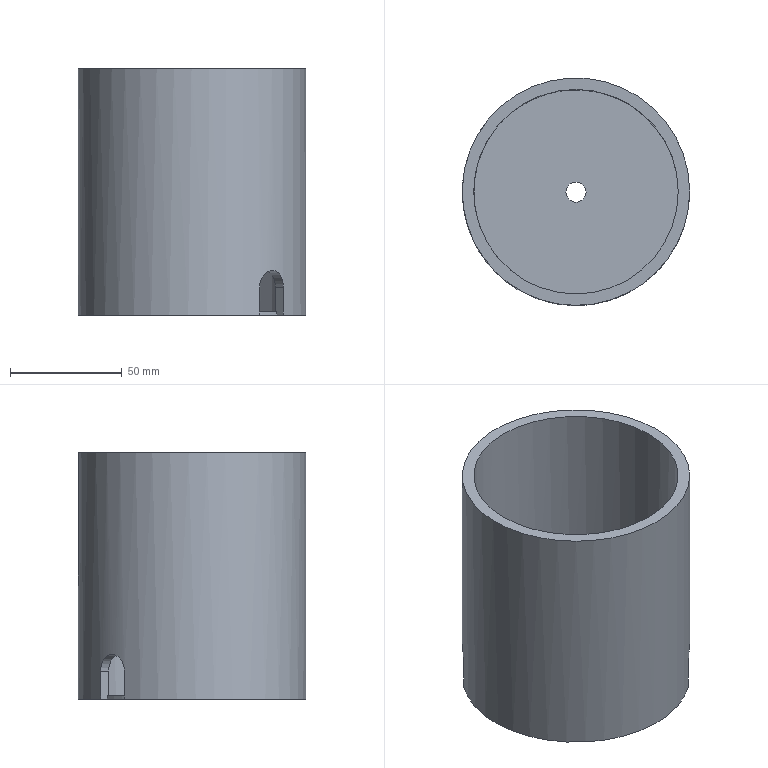Part | NX | features solid 2 | 1 solid | 14 faces | box 101.6 x 101.6 x 110 mm | volume 177690 mm3 | plane 7 | cylinder 7 | commonest cylinder face diameters 15 x2 93.2 x2 9 x1 91.4 x1 101.6 x1
STEP:
#1=CARTESIAN_POINT('',(-1547.218,877.825,-80.));
#2=VERTEX_POINT('',#1);
#3=CARTESIAN_POINT('',(-1550.224,880.831,-80.));
#4=VERTEX_POINT('',#3);
#5=CARTESIAN_POINT('',(-1458.128,788.735,-80.));
#6=DIRECTION('',(-0.7071,0.7071,0.));
#7=VECTOR('',#6,1000.);
#8=LINE('',#5,#7);
#9=EDGE_CURVE('',#2,#4,#8,.T.);
#10=ORIENTED_EDGE('',*,*,#9,.F.);
#11=CARTESIAN_POINT('',(-1547.218,877.825,-78.4));
#12=VERTEX_POINT('',#11);
#13=CARTESIAN_POINT('',(-1547.218,877.825,-78.4));
#14=DIRECTION('',(0.,0.,-1.));
#15=VECTOR('',#14,1000.);
#16=LINE('',#13,#15);
#17=EDGE_CURVE('',#2,#12,#16,.F.);
#18=ORIENTED_EDGE('',*,*,#17,.T.);
#19=CARTESIAN_POINT('',(-1546.573,877.18,-78.4));
#20=VERTEX_POINT('',#19);
#21=CARTESIAN_POINT('',(-1458.128,788.735,-78.4));
#22=DIRECTION('',(-0.7071,0.7071,0.));
#23=VECTOR('',#22,1000.);
#24=LINE('',#21,#23);
#25=EDGE_CURVE('',#20,#12,#24,.T.);
#26=ORIENTED_EDGE('',*,*,#25,.F.);
#27=CARTESIAN_POINT('',(-1546.573,877.18,-67.5));
#28=VERTEX_POINT('',#27);
#29=CARTESIAN_POINT('',(-1546.573,877.18,-80.));
#30=DIRECTION('',(0.,0.,1.));
#31=VECTOR('',#30,1000.);
#32=LINE('',#29,#31);
#33=EDGE_CURVE('',#28,#20,#32,.F.);
#34=ORIENTED_EDGE('',*,*,#33,.F.);
#35=CARTESIAN_POINT('',(-1550.224,880.831,-67.5));
#36=VERTEX_POINT('',#35);
#37=CARTESIAN_POINT('',(-1458.128,788.735,-67.5));
#38=DIRECTION('',(-0.7071,0.7071,0.));
#39=VECTOR('',#38,1000.);
#40=LINE('',#37,#39);
#41=EDGE_CURVE('',#28,#36,#40,.T.);
#42=ORIENTED_EDGE('',*,*,#41,.T.);
#43=CARTESIAN_POINT('',(-1550.224,880.831,-80.));
#44=DIRECTION('',(0.,0.,1.));
#45=VECTOR('',#44,1000.);
#46=LINE('',#43,#45);
#47=EDGE_CURVE('',#36,#4,#46,.F.);
#48=ORIENTED_EDGE('',*,*,#47,.T.);
#49=EDGE_LOOP('',(#10,#18,#26,#34,#42,#48));
#50=FACE_BOUND('',#49,.T.);
#51=CARTESIAN_POINT('',(-1458.128,788.735,-67.5));
#52=DIRECTION('',(-0.7071,-0.7071,0.));
#53=DIRECTION('',(0.,0.,1.));
#54=AXIS2_PLACEMENT_3D('',#51,#52,#53);
#55=PLANE('',#54);
#56=ADVANCED_FACE('',(#50),#55,.T.);
#57=CARTESIAN_POINT('',(-1557.825,867.218,-78.4));
#58=VERTEX_POINT('',#57);
#59=CARTESIAN_POINT('',(-1557.18,866.573,-78.4));
#60=VERTEX_POINT('',#59);
#61=CARTESIAN_POINT('',(-1468.735,778.128,-78.4));
#62=DIRECTION('',(0.7071,-0.7071,0.));
#63=VECTOR('',#62,1000.);
#64=LINE('',#61,#63);
#65=EDGE_CURVE('',#58,#60,#64,.T.);
#66=ORIENTED_EDGE('',*,*,#65,.F.);
#67=CARTESIAN_POINT('',(-1557.825,867.218,-80.));
#68=VERTEX_POINT('',#67);
#69=CARTESIAN_POINT('',(-1557.825,867.218,-78.4));
#70=DIRECTION('',(0.,0.,-1.));
#71=VECTOR('',#70,1000.);
#72=LINE('',#69,#71);
#73=EDGE_CURVE('',#58,#68,#72,.T.);
#74=ORIENTED_EDGE('',*,*,#73,.T.);
#75=CARTESIAN_POINT('',(-1560.831,870.224,-80.));
#76=VERTEX_POINT('',#75);
#77=CARTESIAN_POINT('',(-1468.735,778.128,-80.));
#78=DIRECTION('',(-0.7071,0.7071,0.));
#79=VECTOR('',#78,1000.);
#80=LINE('',#77,#79);
#81=EDGE_CURVE('',#68,#76,#80,.T.);
#82=ORIENTED_EDGE('',*,*,#81,.T.);
#83=CARTESIAN_POINT('',(-1560.831,870.224,-67.5));
#84=VERTEX_POINT('',#83);
#85=CARTESIAN_POINT('',(-1560.831,870.224,-80.));
#86=DIRECTION('',(0.,0.,1.));
#87=VECTOR('',#86,1000.);
#88=LINE('',#85,#87);
#89=EDGE_CURVE('',#76,#84,#88,.T.);
#90=ORIENTED_EDGE('',*,*,#89,.T.);
#91=CARTESIAN_POINT('',(-1557.18,866.573,-67.5));
#92=VERTEX_POINT('',#91);
#93=CARTESIAN_POINT('',(-1468.735,778.128,-67.5));
#94=DIRECTION('',(-0.7071,0.7071,0.));
#95=VECTOR('',#94,1000.);
#96=LINE('',#93,#95);
#97=EDGE_CURVE('',#92,#84,#96,.T.);
#98=ORIENTED_EDGE('',*,*,#97,.F.);
#99=CARTESIAN_POINT('',(-1557.18,866.573,-80.));
#100=DIRECTION('',(0.,0.,1.));
#101=VECTOR('',#100,1000.);
#102=LINE('',#99,#101);
#103=EDGE_CURVE('',#60,#92,#102,.T.);
#104=ORIENTED_EDGE('',*,*,#103,.F.);
#105=EDGE_LOOP('',(#66,#74,#82,#90,#98,#104));
#106=FACE_BOUND('',#105,.T.);
#107=CARTESIAN_POINT('',(-1468.735,778.128,-80.));
#108=DIRECTION('',(0.7071,0.7071,0.));
#109=DIRECTION('',(0.,0.,-1.));
#110=AXIS2_PLACEMENT_3D('',#107,#108,#109);
#111=PLANE('',#110);
#112=ADVANCED_FACE('',(#106),#111,.T.);
#113=CARTESIAN_POINT('',(-1489.776,799.169,-80.));
#114=VERTEX_POINT('',#113);
#115=CARTESIAN_POINT('',(-1492.782,802.175,-80.));
#116=VERTEX_POINT('',#115);
#117=CARTESIAN_POINT('',(-1468.735,778.128,-80.));
#118=DIRECTION('',(-0.7071,0.7071,0.));
#119=VECTOR('',#118,1000.);
#120=LINE('',#117,#119);
#121=EDGE_CURVE('',#114,#116,#120,.T.);
#122=ORIENTED_EDGE('',*,*,#121,.T.);
#123=CARTESIAN_POINT('',(-1492.782,802.175,-78.4));
#124=VERTEX_POINT('',#123);
#125=CARTESIAN_POINT('',(-1492.782,802.175,-78.4));
#126=DIRECTION('',(0.,0.,-1.));
#127=VECTOR('',#126,1000.);
#128=LINE('',#125,#127);
#129=EDGE_CURVE('',#116,#124,#128,.F.);
#130=ORIENTED_EDGE('',*,*,#129,.T.);
#131=CARTESIAN_POINT('',(-1493.427,802.82,-78.4));
#132=VERTEX_POINT('',#131);
#133=CARTESIAN_POINT('',(-1468.735,778.128,-78.4));
#134=DIRECTION('',(0.7071,-0.7071,0.));
#135=VECTOR('',#134,1000.);
#136=LINE('',#133,#135);
#137=EDGE_CURVE('',#132,#124,#136,.T.);
#138=ORIENTED_EDGE('',*,*,#137,.F.);
#139=CARTESIAN_POINT('',(-1493.427,802.82,-67.5));
#140=VERTEX_POINT('',#139);
#141=CARTESIAN_POINT('',(-1493.427,802.82,-80.));
#142=DIRECTION('',(0.,0.,1.));
#143=VECTOR('',#142,1000.);
#144=LINE('',#141,#143);
#145=EDGE_CURVE('',#140,#132,#144,.F.);
#146=ORIENTED_EDGE('',*,*,#145,.F.);
#147=CARTESIAN_POINT('',(-1489.776,799.169,-67.5));
#148=VERTEX_POINT('',#147);
#149=CARTESIAN_POINT('',(-1468.735,778.128,-67.5));
#150=DIRECTION('',(-0.7071,0.7071,0.));
#151=VECTOR('',#150,1000.);
#152=LINE('',#149,#151);
#153=EDGE_CURVE('',#148,#140,#152,.T.);
#154=ORIENTED_EDGE('',*,*,#153,.F.);
#155=CARTESIAN_POINT('',(-1489.776,799.169,-80.));
#156=DIRECTION('',(0.,0.,1.));
#157=VECTOR('',#156,1000.);
#158=LINE('',#155,#157);
#159=EDGE_CURVE('',#148,#114,#158,.F.);
#160=ORIENTED_EDGE('',*,*,#159,.T.);
#161=EDGE_LOOP('',(#122,#130,#138,#146,#154,#160));
#162=FACE_BOUND('',#161,.T.);
#163=CARTESIAN_POINT('',(-1468.735,778.128,-80.));
#164=DIRECTION('',(0.7071,0.7071,0.));
#165=DIRECTION('',(0.,0.,-1.));
#166=AXIS2_PLACEMENT_3D('',#163,#164,#165);
#167=PLANE('',#166);
#168=ADVANCED_FACE('',(#162),#167,.T.);
#169=CARTESIAN_POINT('',(-1482.175,812.782,-78.4));
#170=VERTEX_POINT('',#169);
#171=CARTESIAN_POINT('',(-1482.82,813.427,-78.4));
#172=VERTEX_POINT('',#171);
#173=CARTESIAN_POINT('',(-1458.128,788.735,-78.4));
#174=DIRECTION('',(-0.7071,0.7071,0.));
#175=VECTOR('',#174,1000.);
#176=LINE('',#173,#175);
#177=EDGE_CURVE('',#170,#172,#176,.T.);
#178=ORIENTED_EDGE('',*,*,#177,.F.);
#179=CARTESIAN_POINT('',(-1482.175,812.782,-80.));
#180=VERTEX_POINT('',#179);
#181=CARTESIAN_POINT('',(-1482.175,812.782,-78.4));
#182=DIRECTION('',(0.,0.,-1.));
#183=VECTOR('',#182,1000.);
#184=LINE('',#181,#183);
#185=EDGE_CURVE('',#170,#180,#184,.T.);
#186=ORIENTED_EDGE('',*,*,#185,.T.);
#187=CARTESIAN_POINT('',(-1479.169,809.776,-80.));
#188=VERTEX_POINT('',#187);
#189=CARTESIAN_POINT('',(-1458.128,788.735,-80.));
#190=DIRECTION('',(-0.7071,0.7071,0.));
#191=VECTOR('',#190,1000.);
#192=LINE('',#189,#191);
#193=EDGE_CURVE('',#188,#180,#192,.T.);
#194=ORIENTED_EDGE('',*,*,#193,.F.);
#195=CARTESIAN_POINT('',(-1479.169,809.776,-67.5));
#196=VERTEX_POINT('',#195);
#197=CARTESIAN_POINT('',(-1479.169,809.776,-80.));
#198=DIRECTION('',(0.,0.,1.));
#199=VECTOR('',#198,1000.);
#200=LINE('',#197,#199);
#201=EDGE_CURVE('',#188,#196,#200,.T.);
#202=ORIENTED_EDGE('',*,*,#201,.T.);
#203=CARTESIAN_POINT('',(-1482.82,813.427,-67.5));
#204=VERTEX_POINT('',#203);
#205=CARTESIAN_POINT('',(-1458.128,788.735,-67.5));
#206=DIRECTION('',(-0.7071,0.7071,0.));
#207=VECTOR('',#206,1000.);
#208=LINE('',#205,#207);
#209=EDGE_CURVE('',#196,#204,#208,.T.);
#210=ORIENTED_EDGE('',*,*,#209,.T.);
#211=CARTESIAN_POINT('',(-1482.82,813.427,-80.));
#212=DIRECTION('',(0.,0.,1.));
#213=VECTOR('',#212,1000.);
#214=LINE('',#211,#213);
#215=EDGE_CURVE('',#172,#204,#214,.T.);
#216=ORIENTED_EDGE('',*,*,#215,.F.);
#217=EDGE_LOOP('',(#178,#186,#194,#202,#210,#216));
#218=FACE_BOUND('',#217,.T.);
#219=CARTESIAN_POINT('',(-1458.128,788.735,-67.5));
#220=DIRECTION('',(-0.7071,-0.7071,0.));
#221=DIRECTION('',(0.,0.,1.));
#222=AXIS2_PLACEMENT_3D('',#219,#220,#221);
#223=PLANE('',#222);
#224=ADVANCED_FACE('',(#218),#223,.T.);
#225=CARTESIAN_POINT('',(-1515.5,840.,-80.));
#226=VERTEX_POINT('',#225);
#227=CARTESIAN_POINT('',(-1520.,840.,-80.));
#228=DIRECTION('',(0.,0.,-1.));
#229=DIRECTION('',(1.,0.,0.));
#230=AXIS2_PLACEMENT_3D('',#227,#228,#229);
#231=CIRCLE('',#230,4.5);
#232=EDGE_CURVE('',#226,#226,#231,.F.);
#233=ORIENTED_EDGE('',*,*,#232,.T.);
#234=EDGE_LOOP('',(#233));
#235=FACE_BOUND('',#234,.T.);
#236=CARTESIAN_POINT('',(-1520.,840.,-80.));
#237=DIRECTION('',(0.,0.,1.));
#238=DIRECTION('',(-1.,0.,0.));
#239=AXIS2_PLACEMENT_3D('',#236,#237,#238);
#240=CIRCLE('',#239,46.6);
#241=EDGE_CURVE('',#2,#68,#240,.T.);
#242=ORIENTED_EDGE('',*,*,#241,.F.);
#243=ORIENTED_EDGE('',*,*,#9,.T.);
#244=CARTESIAN_POINT('',(-1520.,840.,-80.));
#245=DIRECTION('',(0.,0.,-1.));
#246=DIRECTION('',(0.7071,0.7071,0.));
#247=AXIS2_PLACEMENT_3D('',#244,#245,#246);
#248=CIRCLE('',#247,50.8);
#249=EDGE_CURVE('',#4,#188,#248,.T.);
#250=ORIENTED_EDGE('',*,*,#249,.T.);
#251=ORIENTED_EDGE('',*,*,#193,.T.);
#252=CARTESIAN_POINT('',(-1520.,840.,-80.));
#253=DIRECTION('',(0.,0.,1.));
#254=DIRECTION('',(-1.,0.,0.));
#255=AXIS2_PLACEMENT_3D('',#252,#253,#254);
#256=CIRCLE('',#255,46.6);
#257=EDGE_CURVE('',#116,#180,#256,.T.);
#258=ORIENTED_EDGE('',*,*,#257,.F.);
#259=ORIENTED_EDGE('',*,*,#121,.F.);
#260=CARTESIAN_POINT('',(-1520.,840.,-80.));
#261=DIRECTION('',(0.,0.,-1.));
#262=DIRECTION('',(0.7071,0.7071,0.));
#263=AXIS2_PLACEMENT_3D('',#260,#261,#262);
#264=CIRCLE('',#263,50.8);
#265=EDGE_CURVE('',#114,#76,#264,.T.);
#266=ORIENTED_EDGE('',*,*,#265,.T.);
#267=ORIENTED_EDGE('',*,*,#81,.F.);
#268=EDGE_LOOP('',(#242,#243,#250,#251,#258,#259,#266,#267));
#269=FACE_BOUND('',#268,.T.);
#270=CARTESIAN_POINT('',(-1520.,840.,-80.));
#271=DIRECTION('',(0.,0.,-1.));
#272=DIRECTION('',(-0.7071,-0.7071,0.));
#273=AXIS2_PLACEMENT_3D('',#270,#271,#272);
#274=PLANE('',#273);
#275=ADVANCED_FACE('',(#235,#269),#274,.T.);
#276=CARTESIAN_POINT('',(-1474.3,840.,30.));
#277=VERTEX_POINT('',#276);
#278=CARTESIAN_POINT('',(-1520.,840.,30.));
#279=DIRECTION('',(0.,0.,-1.));
#280=DIRECTION('',(1.,0.,0.));
#281=AXIS2_PLACEMENT_3D('',#278,#279,#280);
#282=CIRCLE('',#281,45.7);
#283=EDGE_CURVE('',#277,#277,#282,.T.);
#284=ORIENTED_EDGE('',*,*,#283,.F.);
#285=EDGE_LOOP('',(#284));
#286=FACE_BOUND('',#285,.T.);
#287=ORIENTED_EDGE('',*,*,#33,.T.);
#288=CARTESIAN_POINT('',(-1520.,840.,-78.4));
#289=DIRECTION('',(0.,0.,1.));
#290=DIRECTION('',(-1.,0.,0.));
#291=AXIS2_PLACEMENT_3D('',#288,#289,#290);
#292=CIRCLE('',#291,45.7);
#293=EDGE_CURVE('',#20,#172,#292,.F.);
#294=ORIENTED_EDGE('',*,*,#293,.T.);
#295=ORIENTED_EDGE('',*,*,#215,.T.);
#296=CARTESIAN_POINT('',(-1493.427,802.82,-67.5));
#297=CARTESIAN_POINT('',(-1493.427,802.82,-65.54));
#298=CARTESIAN_POINT('',(-1492.058,803.748,-61.623));
#299=CARTESIAN_POINT('',(-1487.576,807.576,-59.188));
#300=CARTESIAN_POINT('',(-1483.745,812.061,-61.626));
#301=CARTESIAN_POINT('',(-1482.82,813.427,-65.541));
#302=CARTESIAN_POINT('',(-1482.82,813.427,-67.5));
#303=B_SPLINE_CURVE_WITH_KNOTS('',3,(#296,#297,#298,#299,#300,#301,#302),.UNSPECIFIED.,.F.,.F.,(4,1,1,1,4),(0.0344,0.04027,0.04614,0.05201,0.05788),.UNSPECIFIED.);
#304=EDGE_CURVE('',#140,#204,#303,.T.);
#305=ORIENTED_EDGE('',*,*,#304,.F.);
#306=ORIENTED_EDGE('',*,*,#145,.T.);
#307=CARTESIAN_POINT('',(-1520.,840.,-78.4));
#308=DIRECTION('',(0.,0.,1.));
#309=DIRECTION('',(-1.,0.,0.));
#310=AXIS2_PLACEMENT_3D('',#307,#308,#309);
#311=CIRCLE('',#310,45.7);
#312=EDGE_CURVE('',#132,#60,#311,.F.);
#313=ORIENTED_EDGE('',*,*,#312,.T.);
#314=ORIENTED_EDGE('',*,*,#103,.T.);
#315=CARTESIAN_POINT('',(-1546.573,877.18,-67.5));
#316=CARTESIAN_POINT('',(-1546.573,877.18,-65.54));
#317=CARTESIAN_POINT('',(-1547.942,876.252,-61.623));
#318=CARTESIAN_POINT('',(-1552.424,872.424,-59.188));
#319=CARTESIAN_POINT('',(-1556.255,867.939,-61.626));
#320=CARTESIAN_POINT('',(-1557.18,866.573,-65.541));
#321=CARTESIAN_POINT('',(-1557.18,866.573,-67.5));
#322=B_SPLINE_CURVE_WITH_KNOTS('',3,(#315,#316,#317,#318,#319,#320,#321),.UNSPECIFIED.,.F.,.F.,(4,1,1,1,4),(0.0344,0.04027,0.04614,0.05201,0.05788),.UNSPECIFIED.);
#323=EDGE_CURVE('',#28,#92,#322,.T.);
#324=ORIENTED_EDGE('',*,*,#323,.F.);
#325=EDGE_LOOP('',(#287,#294,#295,#305,#306,#313,#314,#324));
#326=FACE_BOUND('',#325,.T.);
#327=CARTESIAN_POINT('',(-1520.,840.,-80.));
#328=DIRECTION('',(0.,0.,1.));
#329=DIRECTION('',(0.7071,0.7071,0.));
#330=AXIS2_PLACEMENT_3D('',#327,#328,#329);
#331=CYLINDRICAL_SURFACE('',#330,45.7);
#332=ADVANCED_FACE('',(#286,#326),#331,.F.);
#333=ORIENTED_EDGE('',*,*,#201,.F.);
#334=ORIENTED_EDGE('',*,*,#249,.F.);
#335=ORIENTED_EDGE('',*,*,#47,.F.);
#336=CARTESIAN_POINT('',(-1550.224,880.831,-67.5));
#337=CARTESIAN_POINT('',(-1550.224,880.831,-65.515));
#338=CARTESIAN_POINT('',(-1551.571,879.879,-61.635));
#339=CARTESIAN_POINT('',(-1556.013,876.025,-59.184));
#340=CARTESIAN_POINT('',(-1559.879,871.572,-61.63));
#341=CARTESIAN_POINT('',(-1560.831,870.224,-65.515));
#342=CARTESIAN_POINT('',(-1560.831,870.224,-67.5));
#343=B_SPLINE_CURVE_WITH_KNOTS('',3,(#336,#337,#338,#339,#340,#341,#342),.UNSPECIFIED.,.F.,.F.,(4,1,1,1,4),(0.,0.005869,0.01174,0.01761,0.02347),.UNSPECIFIED.);
#344=EDGE_CURVE('',#36,#84,#343,.T.);
#345=ORIENTED_EDGE('',*,*,#344,.T.);
#346=ORIENTED_EDGE('',*,*,#89,.F.);
#347=ORIENTED_EDGE('',*,*,#265,.F.);
#348=ORIENTED_EDGE('',*,*,#159,.F.);
#349=CARTESIAN_POINT('',(-1489.776,799.169,-67.5));
#350=CARTESIAN_POINT('',(-1489.776,799.169,-65.515));
#351=CARTESIAN_POINT('',(-1488.429,800.121,-61.635));
#352=CARTESIAN_POINT('',(-1483.987,803.975,-59.184));
#353=CARTESIAN_POINT('',(-1480.121,808.428,-61.63));
#354=CARTESIAN_POINT('',(-1479.169,809.776,-65.515));
#355=CARTESIAN_POINT('',(-1479.169,809.776,-67.5));
#356=B_SPLINE_CURVE_WITH_KNOTS('',3,(#349,#350,#351,#352,#353,#354,#355),.UNSPECIFIED.,.F.,.F.,(4,1,1,1,4),(0.,0.005869,0.01174,0.01761,0.02347),.UNSPECIFIED.);
#357=EDGE_CURVE('',#148,#196,#356,.T.);
#358=ORIENTED_EDGE('',*,*,#357,.T.);
#359=EDGE_LOOP('',(#333,#334,#335,#345,#346,#347,#348,#358));
#360=FACE_BOUND('',#359,.T.);
#361=CARTESIAN_POINT('',(-1555.921,804.079,30.));
#362=VERTEX_POINT('',#361);
#363=CARTESIAN_POINT('',(-1520.,840.,30.));
#364=DIRECTION('',(0.,0.,1.));
#365=DIRECTION('',(-0.7071,-0.7071,0.));
#366=AXIS2_PLACEMENT_3D('',#363,#364,#365);
#367=CIRCLE('',#366,50.8);
#368=EDGE_CURVE('',#362,#362,#367,.F.);
#369=ORIENTED_EDGE('',*,*,#368,.T.);
#370=EDGE_LOOP('',(#369));
#371=FACE_BOUND('',#370,.T.);
#372=CARTESIAN_POINT('',(-1520.,840.,-80.));
#373=DIRECTION('',(0.,0.,1.));
#374=DIRECTION('',(0.7071,0.7071,0.));
#375=AXIS2_PLACEMENT_3D('',#372,#373,#374);
#376=CYLINDRICAL_SURFACE('',#375,50.8);
#377=ADVANCED_FACE('',(#360,#371),#376,.T.);
#378=ORIENTED_EDGE('',*,*,#283,.T.);
#379=EDGE_LOOP('',(#378));
#380=FACE_BOUND('',#379,.T.);
#381=ORIENTED_EDGE('',*,*,#368,.F.);
#382=EDGE_LOOP('',(#381));
#383=FACE_BOUND('',#382,.T.);
#384=CARTESIAN_POINT('',(-1520.,840.,30.));
#385=DIRECTION('',(0.,0.,-1.));
#386=DIRECTION('',(-0.7071,-0.7071,0.));
#387=AXIS2_PLACEMENT_3D('',#384,#385,#386);
#388=PLANE('',#387);
#389=ADVANCED_FACE('',(#380,#383),#388,.F.);
#390=ORIENTED_EDGE('',*,*,#41,.F.);
#391=ORIENTED_EDGE('',*,*,#323,.T.);
#392=ORIENTED_EDGE('',*,*,#97,.T.);
#393=ORIENTED_EDGE('',*,*,#344,.F.);
#394=EDGE_LOOP('',(#390,#391,#392,#393));
#395=FACE_BOUND('',#394,.T.);
#396=CARTESIAN_POINT('',(-1463.431,783.431,-67.5));
#397=DIRECTION('',(-0.7071,0.7071,0.));
#398=DIRECTION('',(0.,0.,-1.));
#399=AXIS2_PLACEMENT_3D('',#396,#397,#398);
#400=CYLINDRICAL_SURFACE('',#399,7.5);
#401=ADVANCED_FACE('',(#395),#400,.F.);
#402=ORIENTED_EDGE('',*,*,#153,.T.);
#403=ORIENTED_EDGE('',*,*,#304,.T.);
#404=ORIENTED_EDGE('',*,*,#209,.F.);
#405=ORIENTED_EDGE('',*,*,#357,.F.);
#406=EDGE_LOOP('',(#402,#403,#404,#405));
#407=FACE_BOUND('',#406,.T.);
#408=CARTESIAN_POINT('',(-1463.431,783.431,-67.5));
#409=DIRECTION('',(-0.7071,0.7071,0.));
#410=DIRECTION('',(0.,0.,-1.));
#411=AXIS2_PLACEMENT_3D('',#408,#409,#410);
#412=CYLINDRICAL_SURFACE('',#411,7.5);
#413=ADVANCED_FACE('',(#407),#412,.F.);
#414=ORIENTED_EDGE('',*,*,#17,.F.);
#415=ORIENTED_EDGE('',*,*,#241,.T.);
#416=ORIENTED_EDGE('',*,*,#73,.F.);
#417=CARTESIAN_POINT('',(-1520.,840.,-78.4));
#418=DIRECTION('',(0.,0.,1.));
#419=DIRECTION('',(-1.,0.,0.));
#420=AXIS2_PLACEMENT_3D('',#417,#418,#419);
#421=CIRCLE('',#420,46.6);
#422=EDGE_CURVE('',#12,#58,#421,.T.);
#423=ORIENTED_EDGE('',*,*,#422,.F.);
#424=EDGE_LOOP('',(#414,#415,#416,#423));
#425=FACE_BOUND('',#424,.T.);
#426=CARTESIAN_POINT('',(-1520.,840.,-78.4));
#427=DIRECTION('',(0.,0.,-1.));
#428=DIRECTION('',(1.,0.,0.));
#429=AXIS2_PLACEMENT_3D('',#426,#427,#428);
#430=CYLINDRICAL_SURFACE('',#429,46.6);
#431=ADVANCED_FACE('',(#425),#430,.T.);
#432=ORIENTED_EDGE('',*,*,#129,.F.);
#433=ORIENTED_EDGE('',*,*,#257,.T.);
#434=ORIENTED_EDGE('',*,*,#185,.F.);
#435=CARTESIAN_POINT('',(-1520.,840.,-78.4));
#436=DIRECTION('',(0.,0.,1.));
#437=DIRECTION('',(-1.,0.,0.));
#438=AXIS2_PLACEMENT_3D('',#435,#436,#437);
#439=CIRCLE('',#438,46.6);
#440=EDGE_CURVE('',#124,#170,#439,.T.);
#441=ORIENTED_EDGE('',*,*,#440,.F.);
#442=EDGE_LOOP('',(#432,#433,#434,#441));
#443=FACE_BOUND('',#442,.T.);
#444=CARTESIAN_POINT('',(-1520.,840.,-78.4));
#445=DIRECTION('',(0.,0.,-1.));
#446=DIRECTION('',(1.,0.,0.));
#447=AXIS2_PLACEMENT_3D('',#444,#445,#446);
#448=CYLINDRICAL_SURFACE('',#447,46.6);
#449=ADVANCED_FACE('',(#443),#448,.T.);
#450=CARTESIAN_POINT('',(-1515.5,840.,-78.4));
#451=VERTEX_POINT('',#450);
#452=CARTESIAN_POINT('',(-1520.,840.,-78.4));
#453=DIRECTION('',(0.,0.,-1.));
#454=DIRECTION('',(1.,0.,0.));
#455=AXIS2_PLACEMENT_3D('',#452,#453,#454);
#456=CIRCLE('',#455,4.5);
#457=EDGE_CURVE('',#451,#451,#456,.T.);
#458=ORIENTED_EDGE('',*,*,#457,.T.);
#459=EDGE_LOOP('',(#458));
#460=FACE_BOUND('',#459,.T.);
#461=ORIENTED_EDGE('',*,*,#422,.T.);
#462=ORIENTED_EDGE('',*,*,#65,.T.);
#463=ORIENTED_EDGE('',*,*,#312,.F.);
#464=ORIENTED_EDGE('',*,*,#137,.T.);
#465=ORIENTED_EDGE('',*,*,#440,.T.);
#466=ORIENTED_EDGE('',*,*,#177,.T.);
#467=ORIENTED_EDGE('',*,*,#293,.F.);
#468=ORIENTED_EDGE('',*,*,#25,.T.);
#469=EDGE_LOOP('',(#461,#462,#463,#464,#465,#466,#467,#468));
#470=FACE_BOUND('',#469,.T.);
#471=CARTESIAN_POINT('',(-1520.,840.,-78.4));
#472=DIRECTION('',(0.,0.,1.));
#473=DIRECTION('',(-1.,0.,0.));
#474=AXIS2_PLACEMENT_3D('',#471,#472,#473);
#475=PLANE('',#474);
#476=ADVANCED_FACE('',(#460,#470),#475,.T.);
#477=ORIENTED_EDGE('',*,*,#457,.F.);
#478=EDGE_LOOP('',(#477));
#479=FACE_BOUND('',#478,.T.);
#480=ORIENTED_EDGE('',*,*,#232,.F.);
#481=EDGE_LOOP('',(#480));
#482=FACE_BOUND('',#481,.T.);
#483=CARTESIAN_POINT('',(-1520.,840.,-78.4));
#484=DIRECTION('',(0.,0.,-1.));
#485=DIRECTION('',(1.,0.,0.));
#486=AXIS2_PLACEMENT_3D('',#483,#484,#485);
#487=CYLINDRICAL_SURFACE('',#486,4.5);
#488=ADVANCED_FACE('',(#479,#482),#487,.F.);
#489=CLOSED_SHELL('',(#56,#112,#168,#224,#275,#332,#377,#389,#401,#413,#431,#449,#476,#488));
#490=MANIFOLD_SOLID_BREP('',#489);
#491=(LENGTH_UNIT()NAMED_UNIT(*)SI_UNIT(.MILLI.,.METRE.));
#492=UNCERTAINTY_MEASURE_WITH_UNIT(LENGTH_MEASURE(0.0508),#491,'','');
#493=(NAMED_UNIT(*)PLANE_ANGLE_UNIT()SI_UNIT($,.RADIAN.));
#494=(NAMED_UNIT(*)SI_UNIT($,.STERADIAN.)SOLID_ANGLE_UNIT());
#495=(GEOMETRIC_REPRESENTATION_CONTEXT(3)GLOBAL_UNCERTAINTY_ASSIGNED_CONTEXT((#492))GLOBAL_UNIT_ASSIGNED_CONTEXT((#491,#493,#494))REPRESENTATION_CONTEXT('',''));
#496=ADVANCED_BREP_SHAPE_REPRESENTATION('',(#490),#495);